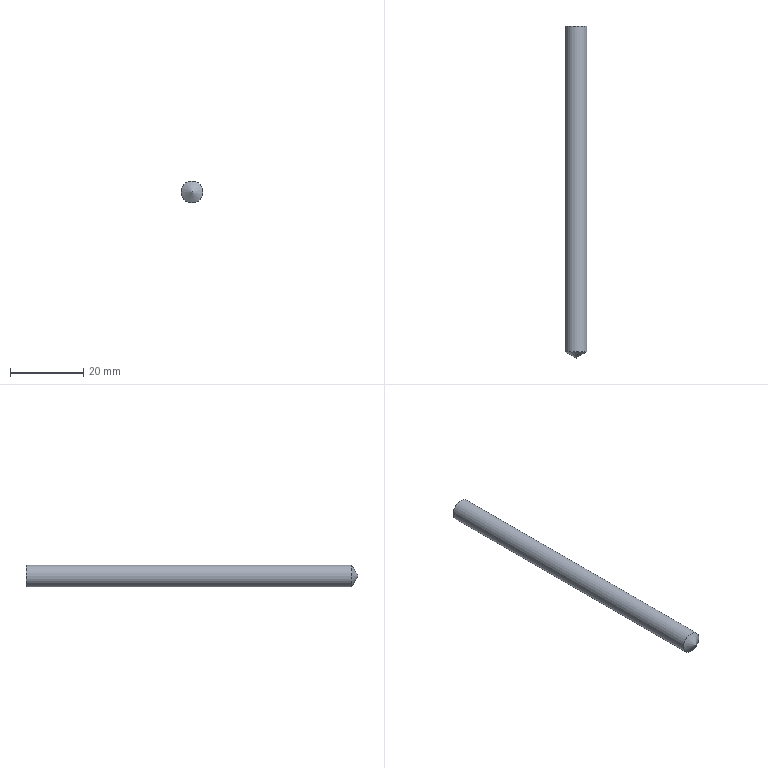Part | NX | features solid 2 | 1 solid | 3 faces | box 6 x 90.732 x 6 mm | volume 2533 mm3 | cylinder 1 | plane 1 | cone 1 | commonest cylinder face diameters 6 x1
STEP:
#1=CARTESIAN_POINT('',(88.,31.,-100.));
#2=VERTEX_POINT('',#1);
#3=CARTESIAN_POINT('',(85.,31.,-100.));
#4=DIRECTION('',(0.,-1.,0.));
#5=DIRECTION('',(1.,0.,0.));
#6=AXIS2_PLACEMENT_3D('',#3,#4,#5);
#7=CIRCLE('',#6,3.);
#8=EDGE_CURVE('',#2,#2,#7,.T.);
#9=ORIENTED_EDGE('',*,*,#8,.F.);
#10=EDGE_LOOP('',(#9));
#11=FACE_BOUND('',#10,.T.);
#12=CARTESIAN_POINT('',(88.,120.,-100.));
#13=VERTEX_POINT('',#12);
#14=CARTESIAN_POINT('',(85.,120.,-100.));
#15=DIRECTION('',(0.,-1.,0.));
#16=DIRECTION('',(1.,0.,0.));
#17=AXIS2_PLACEMENT_3D('',#14,#15,#16);
#18=CIRCLE('',#17,3.);
#19=EDGE_CURVE('',#13,#13,#18,.T.);
#20=ORIENTED_EDGE('',*,*,#19,.T.);
#21=EDGE_LOOP('',(#20));
#22=FACE_BOUND('',#21,.T.);
#23=CARTESIAN_POINT('',(85.,35.,-100.));
#24=DIRECTION('',(0.,1.,0.));
#25=DIRECTION('',(-1.,0.,0.));
#26=AXIS2_PLACEMENT_3D('',#23,#24,#25);
#27=CYLINDRICAL_SURFACE('',#26,3.);
#28=ADVANCED_FACE('',(#11,#22),#27,.T.);
#29=ORIENTED_EDGE('',*,*,#19,.F.);
#30=EDGE_LOOP('',(#29));
#31=FACE_BOUND('',#30,.T.);
#32=CARTESIAN_POINT('',(85.,120.,-100.));
#33=DIRECTION('',(0.,-1.,0.));
#34=DIRECTION('',(1.,0.,0.));
#35=AXIS2_PLACEMENT_3D('',#32,#33,#34);
#36=PLANE('',#35);
#37=ADVANCED_FACE('',(#31),#36,.F.);
#38=ORIENTED_EDGE('',*,*,#8,.T.);
#39=EDGE_LOOP('',(#38));
#40=FACE_BOUND('',#39,.T.);
#41=CARTESIAN_POINT('',(85.,29.268,-100.));
#42=VERTEX_POINT('',#41);
#43=VERTEX_LOOP('',#42);
#44=FACE_BOUND('',#43,.T.);
#45=CARTESIAN_POINT('',(85.,29.268,-100.));
#46=DIRECTION('',(0.,1.,0.));
#47=DIRECTION('',(-1.,0.,0.));
#48=AXIS2_PLACEMENT_3D('',#45,#46,#47);
#49=CONICAL_SURFACE('',#48,0.,1.047);
#50=ADVANCED_FACE('',(#40,#44),#49,.T.);
#51=CLOSED_SHELL('',(#28,#37,#50));
#52=MANIFOLD_SOLID_BREP('',#51);
#53=(LENGTH_UNIT()NAMED_UNIT(*)SI_UNIT(.MILLI.,.METRE.));
#54=UNCERTAINTY_MEASURE_WITH_UNIT(LENGTH_MEASURE(0.00001),#53,'','');
#55=(NAMED_UNIT(*)PLANE_ANGLE_UNIT()SI_UNIT($,.RADIAN.));
#56=(NAMED_UNIT(*)SI_UNIT($,.STERADIAN.)SOLID_ANGLE_UNIT());
#57=(GEOMETRIC_REPRESENTATION_CONTEXT(3)GLOBAL_UNCERTAINTY_ASSIGNED_CONTEXT((#54))GLOBAL_UNIT_ASSIGNED_CONTEXT((#53,#55,#56))REPRESENTATION_CONTEXT('',''));
#58=ADVANCED_BREP_SHAPE_REPRESENTATION('',(#52),#57);